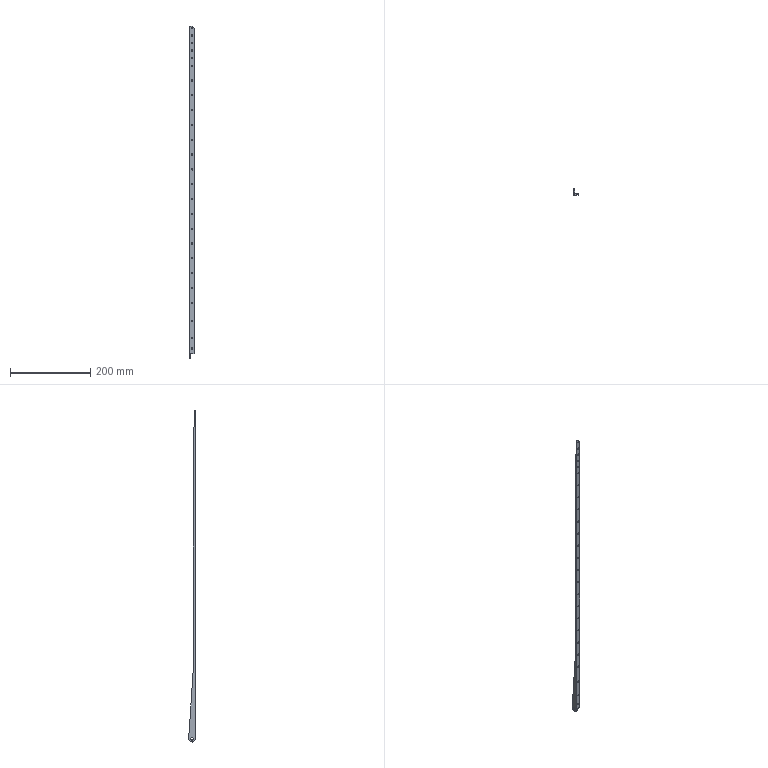Part | SolidWorks | features BaseBody 1 | 1 solid | 66 faces | box 10 x 16 x 829 mm | volume 18614 mm3 | cylinder 54 | plane 12 | commonest cylinder face diameters 3.2 x50 6.35 x2 16 x2